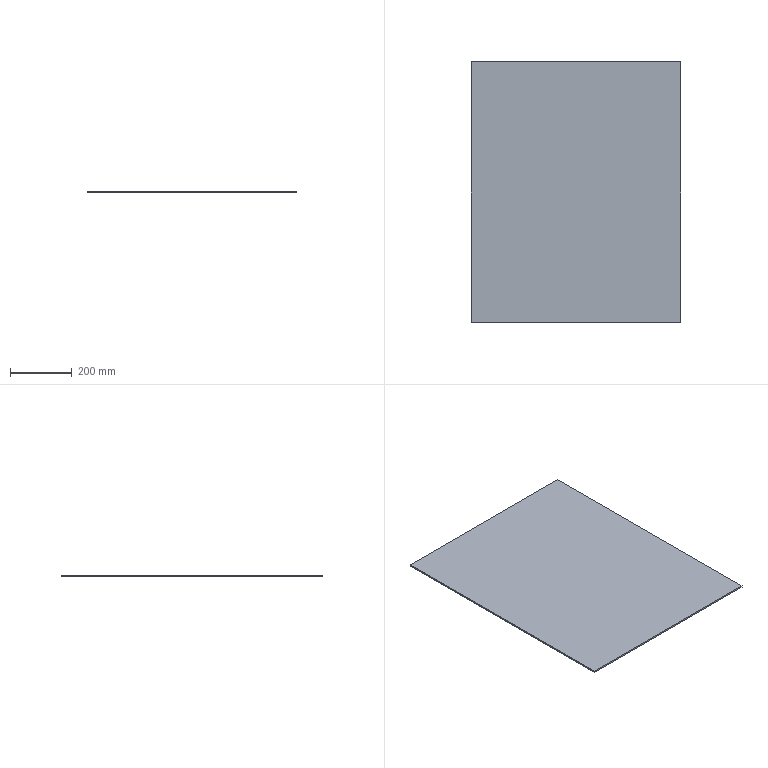Part | SolidWorks | features Extrusion 1, HoleWzd 1 | 1 solid | 6 faces | box 676 x 842 x 5 mm | volume 2845960 mm3 | plane 6
STEP:
#1=CARTESIAN_POINT('',(338.,-421.,0.));
#2=VERTEX_POINT('',#1);
#3=CARTESIAN_POINT('',(338.,421.,0.));
#4=VERTEX_POINT('',#3);
#5=CARTESIAN_POINT('',(338.,421.,0.));
#6=DIRECTION('',(0.,1.,0.));
#7=VECTOR('',#6,1000.);
#8=LINE('',#5,#7);
#9=EDGE_CURVE('',#2,#4,#8,.T.);
#10=ORIENTED_EDGE('',*,*,#9,.T.);
#11=CARTESIAN_POINT('',(338.,421.,5.));
#12=VERTEX_POINT('',#11);
#13=CARTESIAN_POINT('',(338.,421.,5.));
#14=DIRECTION('',(0.,0.,-1.));
#15=VECTOR('',#14,1000.);
#16=LINE('',#13,#15);
#17=EDGE_CURVE('',#12,#4,#16,.T.);
#18=ORIENTED_EDGE('',*,*,#17,.F.);
#19=CARTESIAN_POINT('',(338.,-421.,5.));
#20=VERTEX_POINT('',#19);
#21=CARTESIAN_POINT('',(338.,421.,5.));
#22=DIRECTION('',(0.,1.,0.));
#23=VECTOR('',#22,1000.);
#24=LINE('',#21,#23);
#25=EDGE_CURVE('',#20,#12,#24,.T.);
#26=ORIENTED_EDGE('',*,*,#25,.F.);
#27=CARTESIAN_POINT('',(338.,-421.,5.));
#28=DIRECTION('',(0.,0.,-1.));
#29=VECTOR('',#28,1000.);
#30=LINE('',#27,#29);
#31=EDGE_CURVE('',#20,#2,#30,.T.);
#32=ORIENTED_EDGE('',*,*,#31,.T.);
#33=EDGE_LOOP('',(#10,#18,#26,#32));
#34=FACE_OUTER_BOUND('',#33,.T.);
#35=CARTESIAN_POINT('',(338.,421.,5.));
#36=DIRECTION('',(-1.,0.,0.));
#37=DIRECTION('',(0.,-1.,0.));
#38=AXIS2_PLACEMENT_3D('',#35,#36,#37);
#39=PLANE('',#38);
#40=ADVANCED_FACE('',(#34),#39,.F.);
#41=CARTESIAN_POINT('',(-338.,421.,0.));
#42=VERTEX_POINT('',#41);
#43=CARTESIAN_POINT('',(-338.,421.,0.));
#44=DIRECTION('',(-1.,0.,0.));
#45=VECTOR('',#44,1000.);
#46=LINE('',#43,#45);
#47=EDGE_CURVE('',#4,#42,#46,.T.);
#48=ORIENTED_EDGE('',*,*,#47,.T.);
#49=CARTESIAN_POINT('',(-338.,421.,5.));
#50=VERTEX_POINT('',#49);
#51=CARTESIAN_POINT('',(-338.,421.,5.));
#52=DIRECTION('',(0.,0.,-1.));
#53=VECTOR('',#52,1000.);
#54=LINE('',#51,#53);
#55=EDGE_CURVE('',#50,#42,#54,.T.);
#56=ORIENTED_EDGE('',*,*,#55,.F.);
#57=CARTESIAN_POINT('',(-338.,421.,5.));
#58=DIRECTION('',(-1.,0.,0.));
#59=VECTOR('',#58,1000.);
#60=LINE('',#57,#59);
#61=EDGE_CURVE('',#12,#50,#60,.T.);
#62=ORIENTED_EDGE('',*,*,#61,.F.);
#63=ORIENTED_EDGE('',*,*,#17,.T.);
#64=EDGE_LOOP('',(#48,#56,#62,#63));
#65=FACE_OUTER_BOUND('',#64,.T.);
#66=CARTESIAN_POINT('',(-338.,421.,5.));
#67=DIRECTION('',(0.,-1.,0.));
#68=DIRECTION('',(0.,0.,-1.));
#69=AXIS2_PLACEMENT_3D('',#66,#67,#68);
#70=PLANE('',#69);
#71=ADVANCED_FACE('',(#65),#70,.F.);
#72=CARTESIAN_POINT('',(-338.,-421.,0.));
#73=VERTEX_POINT('',#72);
#74=CARTESIAN_POINT('',(-338.,421.,0.));
#75=DIRECTION('',(0.,-1.,0.));
#76=VECTOR('',#75,1000.);
#77=LINE('',#74,#76);
#78=EDGE_CURVE('',#42,#73,#77,.T.);
#79=ORIENTED_EDGE('',*,*,#78,.T.);
#80=CARTESIAN_POINT('',(-338.,-421.,5.));
#81=VERTEX_POINT('',#80);
#82=CARTESIAN_POINT('',(-338.,-421.,5.));
#83=DIRECTION('',(0.,0.,-1.));
#84=VECTOR('',#83,1000.);
#85=LINE('',#82,#84);
#86=EDGE_CURVE('',#81,#73,#85,.T.);
#87=ORIENTED_EDGE('',*,*,#86,.F.);
#88=CARTESIAN_POINT('',(-338.,421.,5.));
#89=DIRECTION('',(0.,-1.,0.));
#90=VECTOR('',#89,1000.);
#91=LINE('',#88,#90);
#92=EDGE_CURVE('',#50,#81,#91,.T.);
#93=ORIENTED_EDGE('',*,*,#92,.F.);
#94=ORIENTED_EDGE('',*,*,#55,.T.);
#95=EDGE_LOOP('',(#79,#87,#93,#94));
#96=FACE_OUTER_BOUND('',#95,.T.);
#97=CARTESIAN_POINT('',(-338.,421.,5.));
#98=DIRECTION('',(1.,0.,0.));
#99=DIRECTION('',(0.,1.,0.));
#100=AXIS2_PLACEMENT_3D('',#97,#98,#99);
#101=PLANE('',#100);
#102=ADVANCED_FACE('',(#96),#101,.F.);
#103=CARTESIAN_POINT('',(-338.,-421.,0.));
#104=DIRECTION('',(1.,0.,0.));
#105=VECTOR('',#104,1000.);
#106=LINE('',#103,#105);
#107=EDGE_CURVE('',#73,#2,#106,.T.);
#108=ORIENTED_EDGE('',*,*,#107,.T.);
#109=ORIENTED_EDGE('',*,*,#31,.F.);
#110=CARTESIAN_POINT('',(-338.,-421.,5.));
#111=DIRECTION('',(1.,0.,0.));
#112=VECTOR('',#111,1000.);
#113=LINE('',#110,#112);
#114=EDGE_CURVE('',#81,#20,#113,.T.);
#115=ORIENTED_EDGE('',*,*,#114,.F.);
#116=ORIENTED_EDGE('',*,*,#86,.T.);
#117=EDGE_LOOP('',(#108,#109,#115,#116));
#118=FACE_OUTER_BOUND('',#117,.T.);
#119=CARTESIAN_POINT('',(-338.,-421.,5.));
#120=DIRECTION('',(0.,1.,0.));
#121=DIRECTION('',(0.,0.,1.));
#122=AXIS2_PLACEMENT_3D('',#119,#120,#121);
#123=PLANE('',#122);
#124=ADVANCED_FACE('',(#118),#123,.F.);
#125=ORIENTED_EDGE('',*,*,#25,.T.);
#126=ORIENTED_EDGE('',*,*,#61,.T.);
#127=ORIENTED_EDGE('',*,*,#92,.T.);
#128=ORIENTED_EDGE('',*,*,#114,.T.);
#129=EDGE_LOOP('',(#125,#126,#127,#128));
#130=FACE_OUTER_BOUND('',#129,.T.);
#131=CARTESIAN_POINT('',(0.,0.,5.));
#132=DIRECTION('',(0.,0.,1.));
#133=DIRECTION('',(1.,0.,0.));
#134=AXIS2_PLACEMENT_3D('',#131,#132,#133);
#135=PLANE('',#134);
#136=ADVANCED_FACE('',(#130),#135,.T.);
#137=ORIENTED_EDGE('',*,*,#9,.F.);
#138=ORIENTED_EDGE('',*,*,#107,.F.);
#139=ORIENTED_EDGE('',*,*,#78,.F.);
#140=ORIENTED_EDGE('',*,*,#47,.F.);
#141=EDGE_LOOP('',(#137,#138,#139,#140));
#142=FACE_OUTER_BOUND('',#141,.T.);
#143=CARTESIAN_POINT('',(0.,0.,0.));
#144=DIRECTION('',(0.,0.,1.));
#145=DIRECTION('',(1.,0.,0.));
#146=AXIS2_PLACEMENT_3D('',#143,#144,#145);
#147=PLANE('',#146);
#148=ADVANCED_FACE('',(#142),#147,.F.);
#149=CLOSED_SHELL('',(#40,#71,#102,#124,#136,#148));
#150=MANIFOLD_SOLID_BREP('',#149);
#151=CARTESIAN_POINT('',(0.,0.,0.));
#152=DIRECTION('',(0.,0.,1.));
#153=DIRECTION('',(1.,0.,0.));
#154=AXIS2_PLACEMENT_3D('',#151,#152,#153);
#155=(LENGTH_UNIT()NAMED_UNIT(*)SI_UNIT(.MILLI.,.METRE.));
#156=UNCERTAINTY_MEASURE_WITH_UNIT(LENGTH_MEASURE(0.00001),#155,'','');
#157=(NAMED_UNIT(*)PLANE_ANGLE_UNIT()SI_UNIT($,.RADIAN.));
#158=(NAMED_UNIT(*)SI_UNIT($,.STERADIAN.)SOLID_ANGLE_UNIT());
#159=(GEOMETRIC_REPRESENTATION_CONTEXT(3)GLOBAL_UNCERTAINTY_ASSIGNED_CONTEXT((#156))GLOBAL_UNIT_ASSIGNED_CONTEXT((#155,#157,#158))REPRESENTATION_CONTEXT('',''));
#160=ADVANCED_BREP_SHAPE_REPRESENTATION('',(#150,#154),#159);